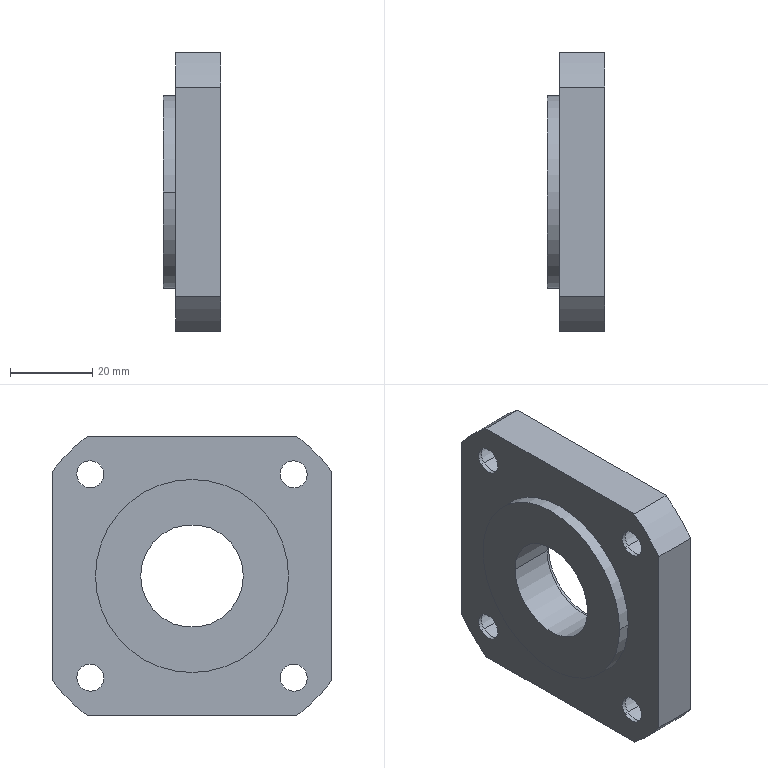Part | NX | 1 solid | 101 faces | box 14 x 68 x 68 mm | volume 41683 mm3 | plane 49 | cylinder 44 | torus 8 | commonest cylinder face diameters 6.6 x8 11 x8 12.9 x8 14 x8 85 x4 25 x2